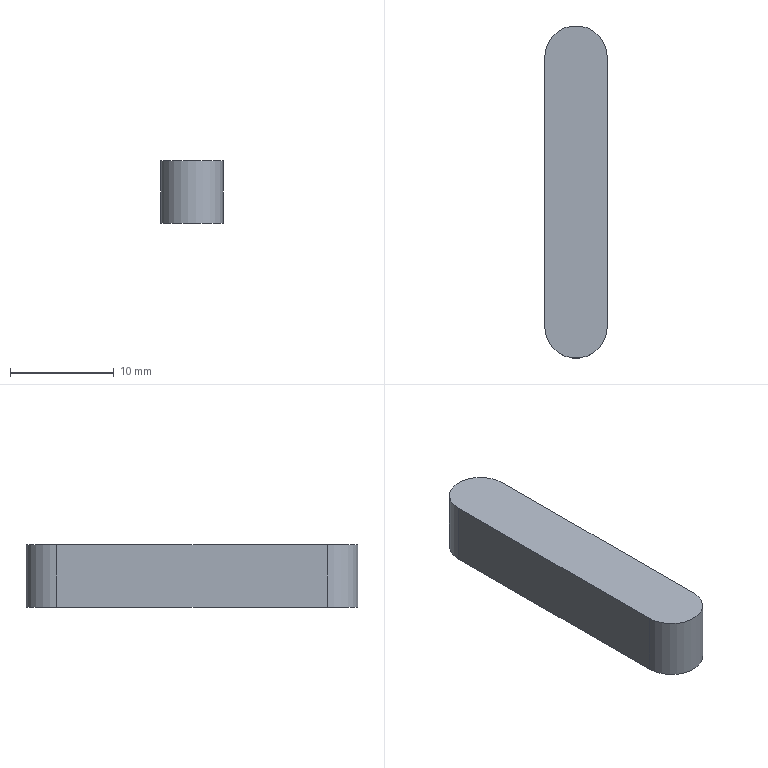Part | SolidWorks | features BaseBody 1 | 1 solid | 6 faces | box 6 x 32 x 6 mm | volume 1106 mm3 | plane 4 | cylinder 2 | commonest cylinder face diameters 6 x2
STEP:
#1=CARTESIAN_POINT('',(3.,0.,0.));
#2=VERTEX_POINT('',#1);
#3=CARTESIAN_POINT('',(-3.,0.,0.));
#4=VERTEX_POINT('',#3);
#5=CARTESIAN_POINT('',(0.,0.,0.));
#6=DIRECTION('',(0.,0.,1.));
#7=DIRECTION('',(1.,0.,0.));
#8=AXIS2_PLACEMENT_3D('',#5,#6,#7);
#9=CIRCLE('',#8,3.);
#10=EDGE_CURVE('',#2,#4,#9,.T.);
#11=ORIENTED_EDGE('',*,*,#10,.F.);
#12=CARTESIAN_POINT('',(3.,-26.,0.));
#13=VERTEX_POINT('',#12);
#14=CARTESIAN_POINT('',(3.,0.,0.));
#15=DIRECTION('',(0.,1.,0.));
#16=VECTOR('',#15,1000.);
#17=LINE('',#14,#16);
#18=EDGE_CURVE('',#13,#2,#17,.T.);
#19=ORIENTED_EDGE('',*,*,#18,.F.);
#20=CARTESIAN_POINT('',(-3.,-26.,0.));
#21=VERTEX_POINT('',#20);
#22=CARTESIAN_POINT('',(0.,-26.,0.));
#23=DIRECTION('',(0.,0.,1.));
#24=DIRECTION('',(1.,0.,0.));
#25=AXIS2_PLACEMENT_3D('',#22,#23,#24);
#26=CIRCLE('',#25,3.);
#27=EDGE_CURVE('',#21,#13,#26,.T.);
#28=ORIENTED_EDGE('',*,*,#27,.F.);
#29=CARTESIAN_POINT('',(-3.,0.,0.));
#30=DIRECTION('',(0.,-1.,0.));
#31=VECTOR('',#30,1000.);
#32=LINE('',#29,#31);
#33=EDGE_CURVE('',#4,#21,#32,.T.);
#34=ORIENTED_EDGE('',*,*,#33,.F.);
#35=EDGE_LOOP('',(#11,#19,#28,#34));
#36=FACE_OUTER_BOUND('',#35,.T.);
#37=CARTESIAN_POINT('',(0.,0.,0.));
#38=DIRECTION('',(0.,0.,1.));
#39=DIRECTION('',(1.,0.,0.));
#40=AXIS2_PLACEMENT_3D('',#37,#38,#39);
#41=PLANE('',#40);
#42=ADVANCED_FACE('',(#36),#41,.F.);
#43=CARTESIAN_POINT('',(3.,0.,6.));
#44=VERTEX_POINT('',#43);
#45=CARTESIAN_POINT('',(-3.,0.,6.));
#46=VERTEX_POINT('',#45);
#47=CARTESIAN_POINT('',(0.,0.,6.));
#48=DIRECTION('',(0.,0.,1.));
#49=DIRECTION('',(1.,0.,0.));
#50=AXIS2_PLACEMENT_3D('',#47,#48,#49);
#51=CIRCLE('',#50,3.);
#52=EDGE_CURVE('',#44,#46,#51,.T.);
#53=ORIENTED_EDGE('',*,*,#52,.T.);
#54=CARTESIAN_POINT('',(-3.,-26.,6.));
#55=VERTEX_POINT('',#54);
#56=CARTESIAN_POINT('',(-3.,0.,6.));
#57=DIRECTION('',(0.,-1.,0.));
#58=VECTOR('',#57,1000.);
#59=LINE('',#56,#58);
#60=EDGE_CURVE('',#46,#55,#59,.T.);
#61=ORIENTED_EDGE('',*,*,#60,.T.);
#62=CARTESIAN_POINT('',(3.,-26.,6.));
#63=VERTEX_POINT('',#62);
#64=CARTESIAN_POINT('',(0.,-26.,6.));
#65=DIRECTION('',(0.,0.,1.));
#66=DIRECTION('',(1.,0.,0.));
#67=AXIS2_PLACEMENT_3D('',#64,#65,#66);
#68=CIRCLE('',#67,3.);
#69=EDGE_CURVE('',#55,#63,#68,.T.);
#70=ORIENTED_EDGE('',*,*,#69,.T.);
#71=CARTESIAN_POINT('',(3.,0.,6.));
#72=DIRECTION('',(0.,1.,0.));
#73=VECTOR('',#72,1000.);
#74=LINE('',#71,#73);
#75=EDGE_CURVE('',#63,#44,#74,.T.);
#76=ORIENTED_EDGE('',*,*,#75,.T.);
#77=EDGE_LOOP('',(#53,#61,#70,#76));
#78=FACE_OUTER_BOUND('',#77,.T.);
#79=CARTESIAN_POINT('',(0.,0.,6.));
#80=DIRECTION('',(0.,0.,1.));
#81=DIRECTION('',(1.,0.,0.));
#82=AXIS2_PLACEMENT_3D('',#79,#80,#81);
#83=PLANE('',#82);
#84=ADVANCED_FACE('',(#78),#83,.T.);
#85=ORIENTED_EDGE('',*,*,#18,.T.);
#86=CARTESIAN_POINT('',(3.,0.,6.));
#87=DIRECTION('',(0.,0.,-1.));
#88=VECTOR('',#87,1000.);
#89=LINE('',#86,#88);
#90=EDGE_CURVE('',#44,#2,#89,.T.);
#91=ORIENTED_EDGE('',*,*,#90,.F.);
#92=ORIENTED_EDGE('',*,*,#75,.F.);
#93=CARTESIAN_POINT('',(3.,-26.,6.));
#94=DIRECTION('',(0.,0.,-1.));
#95=VECTOR('',#94,1000.);
#96=LINE('',#93,#95);
#97=EDGE_CURVE('',#63,#13,#96,.T.);
#98=ORIENTED_EDGE('',*,*,#97,.T.);
#99=EDGE_LOOP('',(#85,#91,#92,#98));
#100=FACE_OUTER_BOUND('',#99,.T.);
#101=CARTESIAN_POINT('',(3.,0.,6.));
#102=DIRECTION('',(-1.,0.,0.));
#103=DIRECTION('',(0.,1.,0.));
#104=AXIS2_PLACEMENT_3D('',#101,#102,#103);
#105=PLANE('',#104);
#106=ADVANCED_FACE('',(#100),#105,.F.);
#107=ORIENTED_EDGE('',*,*,#27,.T.);
#108=ORIENTED_EDGE('',*,*,#97,.F.);
#109=ORIENTED_EDGE('',*,*,#69,.F.);
#110=CARTESIAN_POINT('',(-3.,-26.,6.));
#111=DIRECTION('',(0.,0.,-1.));
#112=VECTOR('',#111,1000.);
#113=LINE('',#110,#112);
#114=EDGE_CURVE('',#55,#21,#113,.T.);
#115=ORIENTED_EDGE('',*,*,#114,.T.);
#116=EDGE_LOOP('',(#107,#108,#109,#115));
#117=FACE_OUTER_BOUND('',#116,.T.);
#118=CARTESIAN_POINT('',(0.,-26.,6.));
#119=DIRECTION('',(0.,0.,-1.));
#120=DIRECTION('',(-1.,0.,0.));
#121=AXIS2_PLACEMENT_3D('',#118,#119,#120);
#122=CYLINDRICAL_SURFACE('',#121,3.);
#123=ADVANCED_FACE('',(#117),#122,.T.);
#124=ORIENTED_EDGE('',*,*,#33,.T.);
#125=ORIENTED_EDGE('',*,*,#114,.F.);
#126=ORIENTED_EDGE('',*,*,#60,.F.);
#127=CARTESIAN_POINT('',(-3.,0.,6.));
#128=DIRECTION('',(0.,0.,-1.));
#129=VECTOR('',#128,1000.);
#130=LINE('',#127,#129);
#131=EDGE_CURVE('',#46,#4,#130,.T.);
#132=ORIENTED_EDGE('',*,*,#131,.T.);
#133=EDGE_LOOP('',(#124,#125,#126,#132));
#134=FACE_OUTER_BOUND('',#133,.T.);
#135=CARTESIAN_POINT('',(-3.,0.,6.));
#136=DIRECTION('',(1.,0.,0.));
#137=DIRECTION('',(0.,0.,1.));
#138=AXIS2_PLACEMENT_3D('',#135,#136,#137);
#139=PLANE('',#138);
#140=ADVANCED_FACE('',(#134),#139,.F.);
#141=ORIENTED_EDGE('',*,*,#10,.T.);
#142=ORIENTED_EDGE('',*,*,#131,.F.);
#143=ORIENTED_EDGE('',*,*,#52,.F.);
#144=ORIENTED_EDGE('',*,*,#90,.T.);
#145=EDGE_LOOP('',(#141,#142,#143,#144));
#146=FACE_OUTER_BOUND('',#145,.T.);
#147=CARTESIAN_POINT('',(0.,0.,6.));
#148=DIRECTION('',(0.,0.,-1.));
#149=DIRECTION('',(-1.,0.,0.));
#150=AXIS2_PLACEMENT_3D('',#147,#148,#149);
#151=CYLINDRICAL_SURFACE('',#150,3.);
#152=ADVANCED_FACE('',(#146),#151,.T.);
#153=CLOSED_SHELL('',(#42,#84,#106,#123,#140,#152));
#154=MANIFOLD_SOLID_BREP('',#153);
#155=CARTESIAN_POINT('',(0.,0.,0.));
#156=DIRECTION('',(0.,0.,1.));
#157=DIRECTION('',(1.,0.,0.));
#158=AXIS2_PLACEMENT_3D('',#155,#156,#157);
#159=(LENGTH_UNIT()NAMED_UNIT(*)SI_UNIT(.MILLI.,.METRE.));
#160=UNCERTAINTY_MEASURE_WITH_UNIT(LENGTH_MEASURE(0.00001),#159,'','');
#161=(NAMED_UNIT(*)PLANE_ANGLE_UNIT()SI_UNIT($,.RADIAN.));
#162=(NAMED_UNIT(*)SI_UNIT($,.STERADIAN.)SOLID_ANGLE_UNIT());
#163=(GEOMETRIC_REPRESENTATION_CONTEXT(3)GLOBAL_UNCERTAINTY_ASSIGNED_CONTEXT((#160))GLOBAL_UNIT_ASSIGNED_CONTEXT((#159,#161,#162))REPRESENTATION_CONTEXT('',''));
#164=ADVANCED_BREP_SHAPE_REPRESENTATION('',(#154,#158),#163);